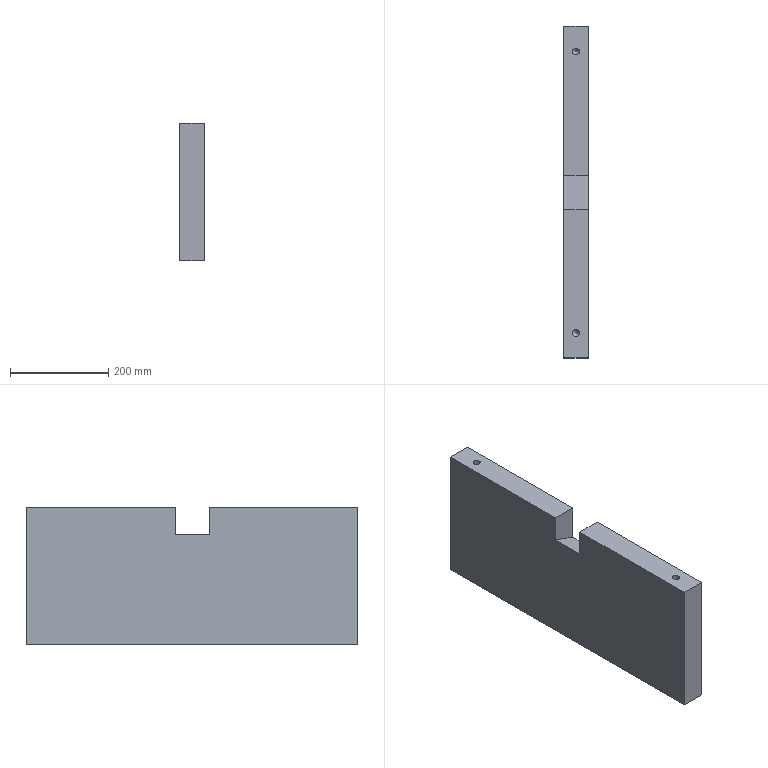Part | NX | features 29 2 | 1 solid | 18 faces | box 50 x 676 x 280.5 mm | volume 9232720 mm3 | plane 10 | cylinder 4 | cone 4 | commonest cylinder face diameters 14.1 x4
STEP:
#1=CARTESIAN_POINT('',(112.05,-287.,-493.5));
#2=VERTEX_POINT('',#1);
#3=CARTESIAN_POINT('',(105.,-287.,-493.5));
#4=DIRECTION('',(0.,0.,1.));
#5=DIRECTION('',(1.,0.,0.));
#6=AXIS2_PLACEMENT_3D('',#3,#4,#5);
#7=CIRCLE('',#6,7.05);
#8=EDGE_CURVE('',#2,#2,#7,.T.);
#9=ORIENTED_EDGE('',*,*,#8,.T.);
#10=EDGE_LOOP('',(#9));
#11=FACE_BOUND('',#10,.T.);
#12=CARTESIAN_POINT('',(130.,-337.,-493.5));
#13=VERTEX_POINT('',#12);
#14=CARTESIAN_POINT('',(130.,339.,-493.5));
#15=VERTEX_POINT('',#14);
#16=CARTESIAN_POINT('',(130.,151.,-493.5));
#17=DIRECTION('',(0.,1.,0.));
#18=VECTOR('',#17,1000.);
#19=LINE('',#16,#18);
#20=EDGE_CURVE('',#13,#15,#19,.T.);
#21=ORIENTED_EDGE('',*,*,#20,.F.);
#22=CARTESIAN_POINT('',(80.,-337.,-493.5));
#23=VERTEX_POINT('',#22);
#24=CARTESIAN_POINT('',(1925.,-337.,-493.5));
#25=DIRECTION('',(-1.,0.,0.));
#26=VECTOR('',#25,1000.);
#27=LINE('',#24,#26);
#28=EDGE_CURVE('',#13,#23,#27,.T.);
#29=ORIENTED_EDGE('',*,*,#28,.T.);
#30=CARTESIAN_POINT('',(80.,339.,-493.5));
#31=VERTEX_POINT('',#30);
#32=CARTESIAN_POINT('',(80.,151.,-493.5));
#33=DIRECTION('',(0.,1.,0.));
#34=VECTOR('',#33,1000.);
#35=LINE('',#32,#34);
#36=EDGE_CURVE('',#23,#31,#35,.T.);
#37=ORIENTED_EDGE('',*,*,#36,.T.);
#38=CARTESIAN_POINT('',(1925.,339.,-493.5));
#39=DIRECTION('',(1.,0.,0.));
#40=VECTOR('',#39,1000.);
#41=LINE('',#38,#40);
#42=EDGE_CURVE('',#31,#15,#41,.T.);
#43=ORIENTED_EDGE('',*,*,#42,.T.);
#44=EDGE_LOOP('',(#21,#29,#37,#43));
#45=FACE_BOUND('',#44,.T.);
#46=CARTESIAN_POINT('',(112.05,287.,-493.5));
#47=VERTEX_POINT('',#46);
#48=CARTESIAN_POINT('',(105.,287.,-493.5));
#49=DIRECTION('',(0.,0.,1.));
#50=DIRECTION('',(1.,0.,0.));
#51=AXIS2_PLACEMENT_3D('',#48,#49,#50);
#52=CIRCLE('',#51,7.05);
#53=EDGE_CURVE('',#47,#47,#52,.T.);
#54=ORIENTED_EDGE('',*,*,#53,.T.);
#55=EDGE_LOOP('',(#54));
#56=FACE_BOUND('',#55,.T.);
#57=CARTESIAN_POINT('',(1925.,0.,-493.5));
#58=DIRECTION('',(0.,0.,-1.));
#59=DIRECTION('',(1.,0.,0.));
#60=AXIS2_PLACEMENT_3D('',#57,#58,#59);
#61=PLANE('',#60);
#62=ADVANCED_FACE('',(#11,#45,#56),#61,.T.);
#63=CARTESIAN_POINT('',(80.,-35.,-213.));
#64=VERTEX_POINT('',#63);
#65=CARTESIAN_POINT('',(130.,-35.,-213.));
#66=VERTEX_POINT('',#65);
#67=CARTESIAN_POINT('',(390.,-35.,-213.));
#68=DIRECTION('',(1.,0.,0.));
#69=VECTOR('',#68,1000.);
#70=LINE('',#67,#69);
#71=EDGE_CURVE('',#64,#66,#70,.T.);
#72=ORIENTED_EDGE('',*,*,#71,.F.);
#73=CARTESIAN_POINT('',(80.,-337.,-213.));
#74=VERTEX_POINT('',#73);
#75=CARTESIAN_POINT('',(80.,151.,-213.));
#76=DIRECTION('',(0.,-1.,0.));
#77=VECTOR('',#76,1000.);
#78=LINE('',#75,#77);
#79=EDGE_CURVE('',#64,#74,#78,.T.);
#80=ORIENTED_EDGE('',*,*,#79,.T.);
#81=CARTESIAN_POINT('',(130.,-337.,-213.));
#82=VERTEX_POINT('',#81);
#83=CARTESIAN_POINT('',(1925.,-337.,-213.));
#84=DIRECTION('',(1.,0.,0.));
#85=VECTOR('',#84,1000.);
#86=LINE('',#83,#85);
#87=EDGE_CURVE('',#74,#82,#86,.T.);
#88=ORIENTED_EDGE('',*,*,#87,.T.);
#89=CARTESIAN_POINT('',(130.,151.,-213.));
#90=DIRECTION('',(0.,-1.,0.));
#91=VECTOR('',#90,1000.);
#92=LINE('',#89,#91);
#93=EDGE_CURVE('',#66,#82,#92,.T.);
#94=ORIENTED_EDGE('',*,*,#93,.F.);
#95=EDGE_LOOP('',(#72,#80,#88,#94));
#96=FACE_BOUND('',#95,.T.);
#97=CARTESIAN_POINT('',(112.05,-287.,-213.));
#98=VERTEX_POINT('',#97);
#99=CARTESIAN_POINT('',(105.,-287.,-213.));
#100=DIRECTION('',(0.,0.,-1.));
#101=DIRECTION('',(1.,0.,0.));
#102=AXIS2_PLACEMENT_3D('',#99,#100,#101);
#103=CIRCLE('',#102,7.05);
#104=EDGE_CURVE('',#98,#98,#103,.T.);
#105=ORIENTED_EDGE('',*,*,#104,.T.);
#106=EDGE_LOOP('',(#105));
#107=FACE_BOUND('',#106,.T.);
#108=CARTESIAN_POINT('',(1925.,0.,-213.));
#109=DIRECTION('',(0.,0.,1.));
#110=DIRECTION('',(-1.,0.,0.));
#111=AXIS2_PLACEMENT_3D('',#108,#109,#110);
#112=PLANE('',#111);
#113=ADVANCED_FACE('',(#96,#107),#112,.T.);
#114=CARTESIAN_POINT('',(80.,35.,-213.));
#115=VERTEX_POINT('',#114);
#116=CARTESIAN_POINT('',(130.,35.,-213.));
#117=VERTEX_POINT('',#116);
#118=CARTESIAN_POINT('',(1925.,35.,-213.));
#119=DIRECTION('',(1.,0.,0.));
#120=VECTOR('',#119,1000.);
#121=LINE('',#118,#120);
#122=EDGE_CURVE('',#115,#117,#121,.T.);
#123=ORIENTED_EDGE('',*,*,#122,.T.);
#124=CARTESIAN_POINT('',(130.,339.,-213.));
#125=VERTEX_POINT('',#124);
#126=CARTESIAN_POINT('',(130.,151.,-213.));
#127=DIRECTION('',(0.,-1.,0.));
#128=VECTOR('',#127,1000.);
#129=LINE('',#126,#128);
#130=EDGE_CURVE('',#125,#117,#129,.T.);
#131=ORIENTED_EDGE('',*,*,#130,.F.);
#132=CARTESIAN_POINT('',(80.,339.,-213.));
#133=VERTEX_POINT('',#132);
#134=CARTESIAN_POINT('',(1925.,339.,-213.));
#135=DIRECTION('',(-1.,0.,0.));
#136=VECTOR('',#135,1000.);
#137=LINE('',#134,#136);
#138=EDGE_CURVE('',#125,#133,#137,.T.);
#139=ORIENTED_EDGE('',*,*,#138,.T.);
#140=CARTESIAN_POINT('',(80.,151.,-213.));
#141=DIRECTION('',(0.,-1.,0.));
#142=VECTOR('',#141,1000.);
#143=LINE('',#140,#142);
#144=EDGE_CURVE('',#133,#115,#143,.T.);
#145=ORIENTED_EDGE('',*,*,#144,.T.);
#146=EDGE_LOOP('',(#123,#131,#139,#145));
#147=FACE_BOUND('',#146,.T.);
#148=CARTESIAN_POINT('',(112.05,287.,-213.));
#149=VERTEX_POINT('',#148);
#150=CARTESIAN_POINT('',(105.,287.,-213.));
#151=DIRECTION('',(0.,0.,-1.));
#152=DIRECTION('',(1.,0.,0.));
#153=AXIS2_PLACEMENT_3D('',#150,#151,#152);
#154=CIRCLE('',#153,7.05);
#155=EDGE_CURVE('',#149,#149,#154,.T.);
#156=ORIENTED_EDGE('',*,*,#155,.T.);
#157=EDGE_LOOP('',(#156));
#158=FACE_BOUND('',#157,.T.);
#159=CARTESIAN_POINT('',(1925.,0.,-213.));
#160=DIRECTION('',(0.,0.,1.));
#161=DIRECTION('',(-1.,0.,0.));
#162=AXIS2_PLACEMENT_3D('',#159,#160,#161);
#163=PLANE('',#162);
#164=ADVANCED_FACE('',(#147,#158),#163,.T.);
#165=ORIENTED_EDGE('',*,*,#28,.F.);
#166=CARTESIAN_POINT('',(130.,-337.,-151.));
#167=DIRECTION('',(0.,0.,-1.));
#168=VECTOR('',#167,1000.);
#169=LINE('',#166,#168);
#170=EDGE_CURVE('',#82,#13,#169,.T.);
#171=ORIENTED_EDGE('',*,*,#170,.F.);
#172=ORIENTED_EDGE('',*,*,#87,.F.);
#173=CARTESIAN_POINT('',(80.,-337.,-68.5));
#174=DIRECTION('',(0.,0.,-1.));
#175=VECTOR('',#174,1000.);
#176=LINE('',#173,#175);
#177=EDGE_CURVE('',#74,#23,#176,.T.);
#178=ORIENTED_EDGE('',*,*,#177,.T.);
#179=EDGE_LOOP('',(#165,#171,#172,#178));
#180=FACE_BOUND('',#179,.T.);
#181=CARTESIAN_POINT('',(157.,-337.,0.));
#182=DIRECTION('',(0.,-1.,0.));
#183=DIRECTION('',(0.,0.,1.));
#184=AXIS2_PLACEMENT_3D('',#181,#182,#183);
#185=PLANE('',#184);
#186=ADVANCED_FACE('',(#180),#185,.T.);
#187=ORIENTED_EDGE('',*,*,#130,.T.);
#188=CARTESIAN_POINT('',(130.,35.,-285.995));
#189=VERTEX_POINT('',#188);
#190=CARTESIAN_POINT('',(130.,35.,-151.));
#191=DIRECTION('',(0.,0.,-1.));
#192=VECTOR('',#191,1000.);
#193=LINE('',#190,#192);
#194=EDGE_CURVE('',#117,#189,#193,.T.);
#195=ORIENTED_EDGE('',*,*,#194,.T.);
#196=CARTESIAN_POINT('',(130.,-35.,-285.995));
#197=VERTEX_POINT('',#196);
#198=CARTESIAN_POINT('',(130.,151.,-285.995));
#199=DIRECTION('',(0.,-1.,0.));
#200=VECTOR('',#199,1000.);
#201=LINE('',#198,#200);
#202=EDGE_CURVE('',#189,#197,#201,.T.);
#203=ORIENTED_EDGE('',*,*,#202,.T.);
#204=CARTESIAN_POINT('',(130.,-35.,-151.));
#205=DIRECTION('',(0.,0.,1.));
#206=VECTOR('',#205,1000.);
#207=LINE('',#204,#206);
#208=EDGE_CURVE('',#197,#66,#207,.T.);
#209=ORIENTED_EDGE('',*,*,#208,.T.);
#210=ORIENTED_EDGE('',*,*,#93,.T.);
#211=ORIENTED_EDGE('',*,*,#170,.T.);
#212=ORIENTED_EDGE('',*,*,#20,.T.);
#213=CARTESIAN_POINT('',(130.,339.,-151.));
#214=DIRECTION('',(0.,0.,1.));
#215=VECTOR('',#214,1000.);
#216=LINE('',#213,#215);
#217=EDGE_CURVE('',#15,#125,#216,.T.);
#218=ORIENTED_EDGE('',*,*,#217,.T.);
#219=EDGE_LOOP('',(#187,#195,#203,#209,#210,#211,#212,#218));
#220=FACE_BOUND('',#219,.T.);
#221=CARTESIAN_POINT('',(130.,151.,-151.));
#222=DIRECTION('',(1.,0.,0.));
#223=DIRECTION('',(0.,0.,-1.));
#224=AXIS2_PLACEMENT_3D('',#221,#222,#223);
#225=PLANE('',#224);
#226=ADVANCED_FACE('',(#220),#225,.T.);
#227=CARTESIAN_POINT('',(80.,35.,-267.796));
#228=VERTEX_POINT('',#227);
#229=CARTESIAN_POINT('',(80.,35.,-68.5));
#230=DIRECTION('',(0.,0.,-1.));
#231=VECTOR('',#230,1000.);
#232=LINE('',#229,#231);
#233=EDGE_CURVE('',#115,#228,#232,.T.);
#234=ORIENTED_EDGE('',*,*,#233,.F.);
#235=ORIENTED_EDGE('',*,*,#144,.F.);
#236=CARTESIAN_POINT('',(80.,339.,-68.5));
#237=DIRECTION('',(0.,0.,1.));
#238=VECTOR('',#237,1000.);
#239=LINE('',#236,#238);
#240=EDGE_CURVE('',#31,#133,#239,.T.);
#241=ORIENTED_EDGE('',*,*,#240,.F.);
#242=ORIENTED_EDGE('',*,*,#36,.F.);
#243=ORIENTED_EDGE('',*,*,#177,.F.);
#244=ORIENTED_EDGE('',*,*,#79,.F.);
#245=CARTESIAN_POINT('',(80.,-35.,-267.796));
#246=VERTEX_POINT('',#245);
#247=CARTESIAN_POINT('',(80.,-35.,-68.5));
#248=DIRECTION('',(0.,0.,1.));
#249=VECTOR('',#248,1000.);
#250=LINE('',#247,#249);
#251=EDGE_CURVE('',#246,#64,#250,.T.);
#252=ORIENTED_EDGE('',*,*,#251,.F.);
#253=CARTESIAN_POINT('',(80.,151.,-267.796));
#254=DIRECTION('',(0.,-1.,0.));
#255=VECTOR('',#254,1000.);
#256=LINE('',#253,#255);
#257=EDGE_CURVE('',#228,#246,#256,.T.);
#258=ORIENTED_EDGE('',*,*,#257,.F.);
#259=EDGE_LOOP('',(#234,#235,#241,#242,#243,#244,#252,#258));
#260=FACE_BOUND('',#259,.T.);
#261=CARTESIAN_POINT('',(80.,151.,-68.5));
#262=DIRECTION('',(1.,0.,0.));
#263=DIRECTION('',(0.,-1.,0.));
#264=AXIS2_PLACEMENT_3D('',#261,#262,#263);
#265=PLANE('',#264);
#266=ADVANCED_FACE('',(#260),#265,.F.);
#267=ORIENTED_EDGE('',*,*,#42,.F.);
#268=ORIENTED_EDGE('',*,*,#240,.T.);
#269=ORIENTED_EDGE('',*,*,#138,.F.);
#270=ORIENTED_EDGE('',*,*,#217,.F.);
#271=EDGE_LOOP('',(#267,#268,#269,#270));
#272=FACE_BOUND('',#271,.T.);
#273=CARTESIAN_POINT('',(42.,339.,0.));
#274=DIRECTION('',(0.,1.,0.));
#275=DIRECTION('',(0.,0.,-1.));
#276=AXIS2_PLACEMENT_3D('',#273,#274,#275);
#277=PLANE('',#276);
#278=ADVANCED_FACE('',(#272),#277,.T.);
#279=ORIENTED_EDGE('',*,*,#122,.F.);
#280=ORIENTED_EDGE('',*,*,#233,.T.);
#281=CARTESIAN_POINT('',(494.006,35.,-418.482));
#282=DIRECTION('',(0.9397,0.,-0.342));
#283=VECTOR('',#282,1000.);
#284=LINE('',#281,#283);
#285=EDGE_CURVE('',#228,#189,#284,.T.);
#286=ORIENTED_EDGE('',*,*,#285,.T.);
#287=ORIENTED_EDGE('',*,*,#194,.F.);
#288=EDGE_LOOP('',(#279,#280,#286,#287));
#289=FACE_BOUND('',#288,.T.);
#290=CARTESIAN_POINT('',(390.,35.,-2110.5));
#291=DIRECTION('',(0.,1.,0.));
#292=DIRECTION('',(0.,0.,1.));
#293=AXIS2_PLACEMENT_3D('',#290,#291,#292);
#294=PLANE('',#293);
#295=ADVANCED_FACE('',(#289),#294,.F.);
#296=ORIENTED_EDGE('',*,*,#285,.F.);
#297=ORIENTED_EDGE('',*,*,#257,.T.);
#298=CARTESIAN_POINT('',(945.97,-35.,-582.984));
#299=DIRECTION('',(0.9397,0.,-0.342));
#300=VECTOR('',#299,1000.);
#301=LINE('',#298,#300);
#302=EDGE_CURVE('',#246,#197,#301,.T.);
#303=ORIENTED_EDGE('',*,*,#302,.T.);
#304=ORIENTED_EDGE('',*,*,#202,.F.);
#305=EDGE_LOOP('',(#296,#297,#303,#304));
#306=FACE_BOUND('',#305,.T.);
#307=CARTESIAN_POINT('',(494.006,-98.921,-418.482));
#308=DIRECTION('',(0.342,0.,0.9397));
#309=DIRECTION('',(0.,1.,0.));
#310=AXIS2_PLACEMENT_3D('',#307,#308,#309);
#311=PLANE('',#310);
#312=ADVANCED_FACE('',(#306),#311,.T.);
#313=ORIENTED_EDGE('',*,*,#302,.F.);
#314=ORIENTED_EDGE('',*,*,#251,.T.);
#315=ORIENTED_EDGE('',*,*,#71,.T.);
#316=ORIENTED_EDGE('',*,*,#208,.F.);
#317=EDGE_LOOP('',(#313,#314,#315,#316));
#318=FACE_BOUND('',#317,.T.);
#319=CARTESIAN_POINT('',(390.,-35.,-2110.5));
#320=DIRECTION('',(0.,-1.,0.));
#321=DIRECTION('',(0.,0.,1.));
#322=AXIS2_PLACEMENT_3D('',#319,#320,#321);
#323=PLANE('',#322);
#324=ADVANCED_FACE('',(#318),#323,.F.);
#325=CARTESIAN_POINT('',(97.95,287.,-249.95));
#326=VERTEX_POINT('',#325);
#327=CARTESIAN_POINT('',(105.,287.,-249.95));
#328=DIRECTION('',(0.,0.,-1.));
#329=DIRECTION('',(-1.,0.,0.));
#330=AXIS2_PLACEMENT_3D('',#327,#328,#329);
#331=CIRCLE('',#330,7.05);
#332=EDGE_CURVE('',#326,#326,#331,.T.);
#333=ORIENTED_EDGE('',*,*,#332,.T.);
#334=EDGE_LOOP('',(#333));
#335=FACE_BOUND('',#334,.T.);
#336=ORIENTED_EDGE('',*,*,#155,.F.);
#337=EDGE_LOOP('',(#336));
#338=FACE_BOUND('',#337,.T.);
#339=CARTESIAN_POINT('',(105.,287.,-213.));
#340=DIRECTION('',(0.,0.,-1.));
#341=DIRECTION('',(-1.,0.,0.));
#342=AXIS2_PLACEMENT_3D('',#339,#340,#341);
#343=CYLINDRICAL_SURFACE('',#342,7.05);
#344=ADVANCED_FACE('',(#335,#338),#343,.F.);
#345=CARTESIAN_POINT('',(105.,287.,-257.));
#346=VERTEX_POINT('',#345);
#347=VERTEX_LOOP('',#346);
#348=FACE_BOUND('',#347,.T.);
#349=ORIENTED_EDGE('',*,*,#332,.F.);
#350=EDGE_LOOP('',(#349));
#351=FACE_BOUND('',#350,.T.);
#352=CARTESIAN_POINT('',(105.,287.,-249.95));
#353=DIRECTION('',(0.,0.,1.));
#354=DIRECTION('',(-1.,0.,0.));
#355=AXIS2_PLACEMENT_3D('',#352,#353,#354);
#356=CONICAL_SURFACE('',#355,7.05,0.7854);
#357=ADVANCED_FACE('',(#348,#351),#356,.F.);
#358=CARTESIAN_POINT('',(97.95,-287.,-249.95));
#359=VERTEX_POINT('',#358);
#360=CARTESIAN_POINT('',(105.,-287.,-249.95));
#361=DIRECTION('',(0.,0.,-1.));
#362=DIRECTION('',(-1.,0.,0.));
#363=AXIS2_PLACEMENT_3D('',#360,#361,#362);
#364=CIRCLE('',#363,7.05);
#365=EDGE_CURVE('',#359,#359,#364,.T.);
#366=ORIENTED_EDGE('',*,*,#365,.T.);
#367=EDGE_LOOP('',(#366));
#368=FACE_BOUND('',#367,.T.);
#369=ORIENTED_EDGE('',*,*,#104,.F.);
#370=EDGE_LOOP('',(#369));
#371=FACE_BOUND('',#370,.T.);
#372=CARTESIAN_POINT('',(105.,-287.,-213.));
#373=DIRECTION('',(0.,0.,-1.));
#374=DIRECTION('',(-1.,0.,0.));
#375=AXIS2_PLACEMENT_3D('',#372,#373,#374);
#376=CYLINDRICAL_SURFACE('',#375,7.05);
#377=ADVANCED_FACE('',(#368,#371),#376,.F.);
#378=CARTESIAN_POINT('',(105.,-287.,-257.));
#379=VERTEX_POINT('',#378);
#380=VERTEX_LOOP('',#379);
#381=FACE_BOUND('',#380,.T.);
#382=ORIENTED_EDGE('',*,*,#365,.F.);
#383=EDGE_LOOP('',(#382));
#384=FACE_BOUND('',#383,.T.);
#385=CARTESIAN_POINT('',(105.,-287.,-249.95));
#386=DIRECTION('',(0.,0.,1.));
#387=DIRECTION('',(-1.,0.,0.));
#388=AXIS2_PLACEMENT_3D('',#385,#386,#387);
#389=CONICAL_SURFACE('',#388,7.05,0.7854);
#390=ADVANCED_FACE('',(#381,#384),#389,.F.);
#391=CARTESIAN_POINT('',(112.05,-287.,-456.55));
#392=VERTEX_POINT('',#391);
#393=CARTESIAN_POINT('',(105.,-287.,-456.55));
#394=DIRECTION('',(0.,0.,1.));
#395=DIRECTION('',(1.,0.,0.));
#396=AXIS2_PLACEMENT_3D('',#393,#394,#395);
#397=CIRCLE('',#396,7.05);
#398=EDGE_CURVE('',#392,#392,#397,.T.);
#399=ORIENTED_EDGE('',*,*,#398,.T.);
#400=EDGE_LOOP('',(#399));
#401=FACE_BOUND('',#400,.T.);
#402=ORIENTED_EDGE('',*,*,#8,.F.);
#403=EDGE_LOOP('',(#402));
#404=FACE_BOUND('',#403,.T.);
#405=CARTESIAN_POINT('',(105.,-287.,-493.5));
#406=DIRECTION('',(0.,0.,1.));
#407=DIRECTION('',(-1.,0.,0.));
#408=AXIS2_PLACEMENT_3D('',#405,#406,#407);
#409=CYLINDRICAL_SURFACE('',#408,7.05);
#410=ADVANCED_FACE('',(#401,#404),#409,.F.);
#411=CARTESIAN_POINT('',(105.,-287.,-449.5));
#412=VERTEX_POINT('',#411);
#413=VERTEX_LOOP('',#412);
#414=FACE_BOUND('',#413,.T.);
#415=ORIENTED_EDGE('',*,*,#398,.F.);
#416=EDGE_LOOP('',(#415));
#417=FACE_BOUND('',#416,.T.);
#418=CARTESIAN_POINT('',(105.,-287.,-456.55));
#419=DIRECTION('',(0.,0.,-1.));
#420=DIRECTION('',(1.,0.,0.));
#421=AXIS2_PLACEMENT_3D('',#418,#419,#420);
#422=CONICAL_SURFACE('',#421,7.05,0.7854);
#423=ADVANCED_FACE('',(#414,#417),#422,.F.);
#424=CARTESIAN_POINT('',(112.05,287.,-456.55));
#425=VERTEX_POINT('',#424);
#426=CARTESIAN_POINT('',(105.,287.,-456.55));
#427=DIRECTION('',(0.,0.,1.));
#428=DIRECTION('',(1.,0.,0.));
#429=AXIS2_PLACEMENT_3D('',#426,#427,#428);
#430=CIRCLE('',#429,7.05);
#431=EDGE_CURVE('',#425,#425,#430,.T.);
#432=ORIENTED_EDGE('',*,*,#431,.T.);
#433=EDGE_LOOP('',(#432));
#434=FACE_BOUND('',#433,.T.);
#435=ORIENTED_EDGE('',*,*,#53,.F.);
#436=EDGE_LOOP('',(#435));
#437=FACE_BOUND('',#436,.T.);
#438=CARTESIAN_POINT('',(105.,287.,-493.5));
#439=DIRECTION('',(0.,0.,1.));
#440=DIRECTION('',(-1.,0.,0.));
#441=AXIS2_PLACEMENT_3D('',#438,#439,#440);
#442=CYLINDRICAL_SURFACE('',#441,7.05);
#443=ADVANCED_FACE('',(#434,#437),#442,.F.);
#444=CARTESIAN_POINT('',(105.,287.,-449.5));
#445=VERTEX_POINT('',#444);
#446=VERTEX_LOOP('',#445);
#447=FACE_BOUND('',#446,.T.);
#448=ORIENTED_EDGE('',*,*,#431,.F.);
#449=EDGE_LOOP('',(#448));
#450=FACE_BOUND('',#449,.T.);
#451=CARTESIAN_POINT('',(105.,287.,-456.55));
#452=DIRECTION('',(0.,0.,-1.));
#453=DIRECTION('',(1.,0.,0.));
#454=AXIS2_PLACEMENT_3D('',#451,#452,#453);
#455=CONICAL_SURFACE('',#454,7.05,0.7854);
#456=ADVANCED_FACE('',(#447,#450),#455,.F.);
#457=CLOSED_SHELL('',(#62,#113,#164,#186,#226,#266,#278,#295,#312,#324,#344,#357,#377,#390,#410,#423,#443,#456));
#458=MANIFOLD_SOLID_BREP('',#457);
#459=(LENGTH_UNIT()NAMED_UNIT(*)SI_UNIT(.MILLI.,.METRE.));
#460=UNCERTAINTY_MEASURE_WITH_UNIT(LENGTH_MEASURE(0.00001),#459,'','');
#461=(NAMED_UNIT(*)PLANE_ANGLE_UNIT()SI_UNIT($,.RADIAN.));
#462=(NAMED_UNIT(*)SI_UNIT($,.STERADIAN.)SOLID_ANGLE_UNIT());
#463=(GEOMETRIC_REPRESENTATION_CONTEXT(3)GLOBAL_UNCERTAINTY_ASSIGNED_CONTEXT((#460))GLOBAL_UNIT_ASSIGNED_CONTEXT((#459,#461,#462))REPRESENTATION_CONTEXT('',''));
#464=ADVANCED_BREP_SHAPE_REPRESENTATION('',(#458),#463);